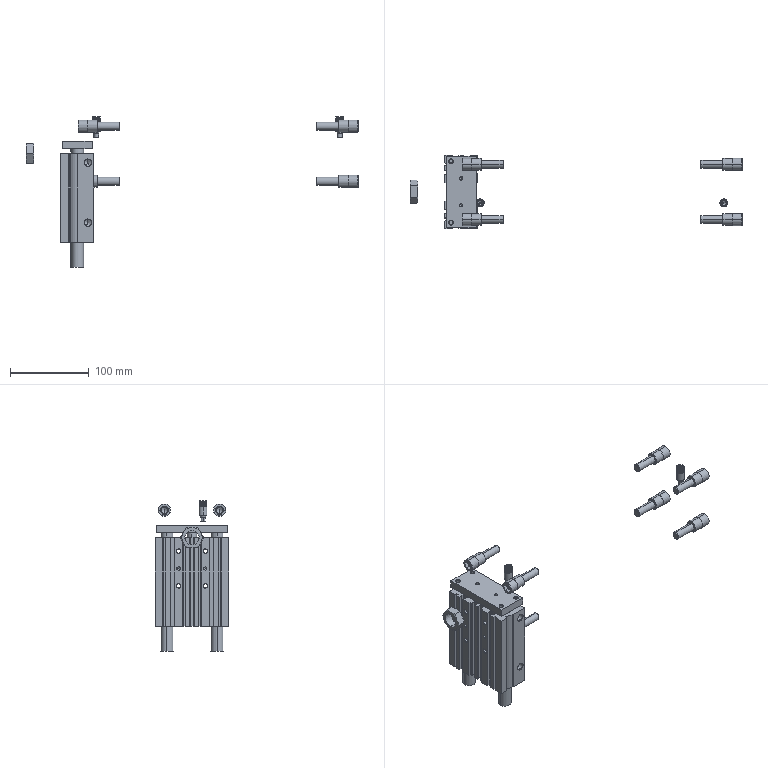Part | SolidWorks | 15 solids | 791 faces | box 421 x 93 x 190.924 mm | volume 447308 mm3 | plane 329 | cone 232 | cylinder 194 | spline 36 | commonest cylinder face diameters 10 x28 4.917 x24 4 x18 8.376 x16 15 x16 15.5 x16